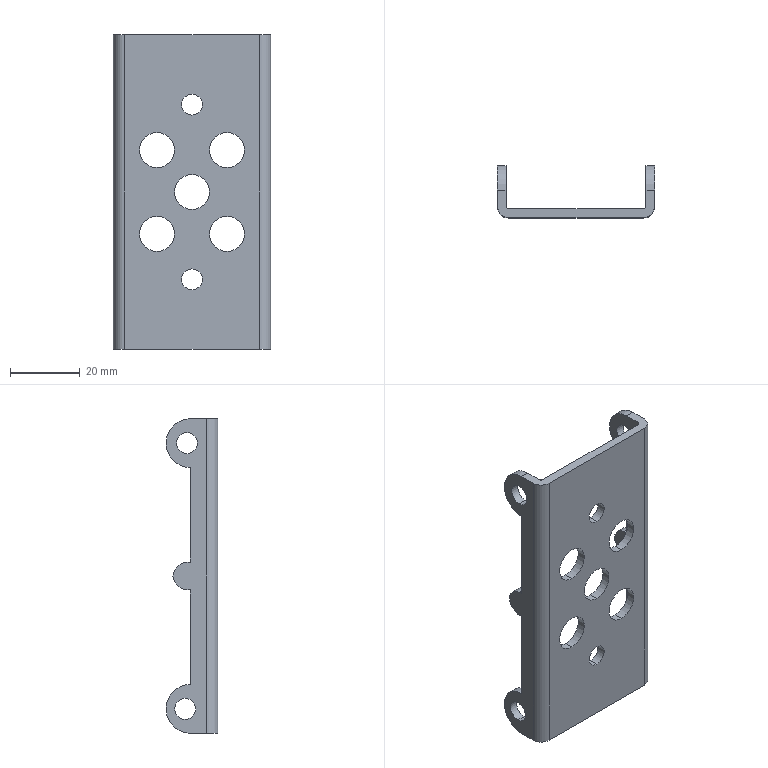Part | SolidWorks | features HoleWzd 4, Fillet 2, ICE 2, Extrusion 1 | 1 solid | 50 faces | box 45 x 14.855 x 90 mm | volume 11672 mm3 | cylinder 34 | plane 16 | commonest cylinder face diameters 6 x12 10 x10 9.055 x4 14 x4 1.473 x2 6.473 x2